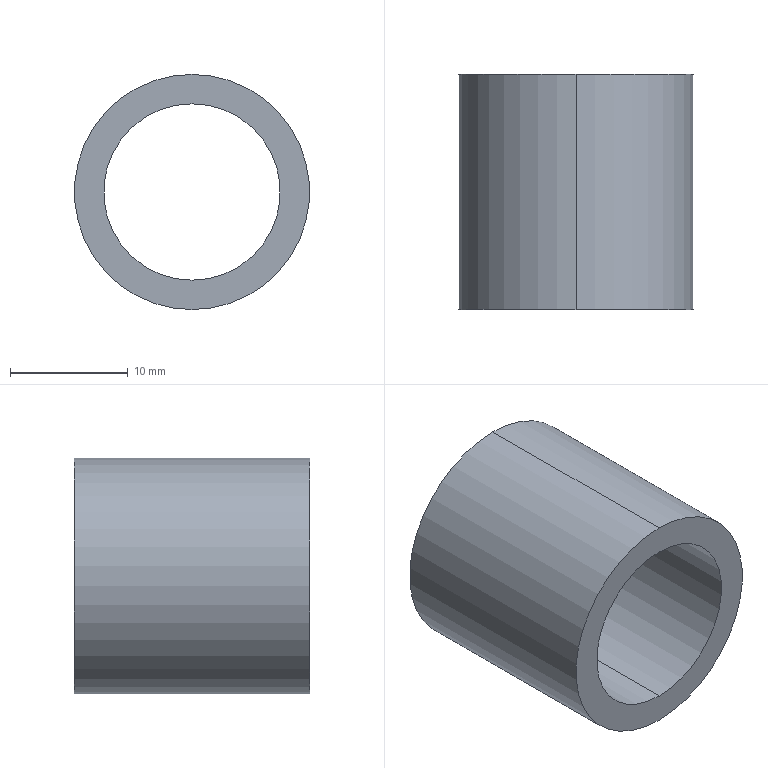Part | SolidWorks | features Extrusion 1 | 1 solid | 6 faces | box 20 x 20 x 20 mm | volume 2749 mm3 | cylinder 4 | plane 2 | commonest cylinder face diameters 15 x2 20 x2
STEP:
#1=CARTESIAN_POINT('',(0.,10.,-7.5));
#2=VERTEX_POINT('',#1);
#3=CARTESIAN_POINT('',(0.,10.,7.5));
#4=VERTEX_POINT('',#3);
#5=CARTESIAN_POINT('',(0.,10.,0.));
#6=DIRECTION('',(0.,1.,0.));
#7=DIRECTION('',(0.,0.,1.));
#8=AXIS2_PLACEMENT_3D('',#5,#6,#7);
#9=CIRCLE('',#8,7.5);
#10=EDGE_CURVE('',#2,#4,#9,.T.);
#11=ORIENTED_EDGE('',*,*,#10,.T.);
#12=CARTESIAN_POINT('',(0.,-10.,7.5));
#13=VERTEX_POINT('',#12);
#14=CARTESIAN_POINT('',(0.,10.,7.5));
#15=DIRECTION('',(0.,-1.,0.));
#16=VECTOR('',#15,1000.);
#17=LINE('',#14,#16);
#18=EDGE_CURVE('',#4,#13,#17,.T.);
#19=ORIENTED_EDGE('',*,*,#18,.T.);
#20=CARTESIAN_POINT('',(0.,-10.,-7.5));
#21=VERTEX_POINT('',#20);
#22=CARTESIAN_POINT('',(0.,-10.,0.));
#23=DIRECTION('',(0.,1.,0.));
#24=DIRECTION('',(0.,0.,1.));
#25=AXIS2_PLACEMENT_3D('',#22,#23,#24);
#26=CIRCLE('',#25,7.5);
#27=EDGE_CURVE('',#21,#13,#26,.T.);
#28=ORIENTED_EDGE('',*,*,#27,.F.);
#29=CARTESIAN_POINT('',(0.,10.,-7.5));
#30=DIRECTION('',(0.,-1.,0.));
#31=VECTOR('',#30,1000.);
#32=LINE('',#29,#31);
#33=EDGE_CURVE('',#2,#21,#32,.T.);
#34=ORIENTED_EDGE('',*,*,#33,.F.);
#35=EDGE_LOOP('',(#11,#19,#28,#34));
#36=FACE_OUTER_BOUND('',#35,.T.);
#37=CARTESIAN_POINT('',(0.,10.,0.));
#38=DIRECTION('',(0.,-1.,0.));
#39=DIRECTION('',(0.,0.,-1.));
#40=AXIS2_PLACEMENT_3D('',#37,#38,#39);
#41=CYLINDRICAL_SURFACE('',#40,7.5);
#42=ADVANCED_FACE('',(#36),#41,.F.);
#43=CARTESIAN_POINT('',(0.,10.,10.));
#44=VERTEX_POINT('',#43);
#45=CARTESIAN_POINT('',(0.,10.,-10.));
#46=VERTEX_POINT('',#45);
#47=CARTESIAN_POINT('',(0.,10.,0.));
#48=DIRECTION('',(0.,1.,0.));
#49=DIRECTION('',(0.,0.,1.));
#50=AXIS2_PLACEMENT_3D('',#47,#48,#49);
#51=CIRCLE('',#50,10.);
#52=EDGE_CURVE('',#44,#46,#51,.T.);
#53=ORIENTED_EDGE('',*,*,#52,.F.);
#54=CARTESIAN_POINT('',(0.,-10.,10.));
#55=VERTEX_POINT('',#54);
#56=CARTESIAN_POINT('',(0.,10.,10.));
#57=DIRECTION('',(0.,-1.,0.));
#58=VECTOR('',#57,1000.);
#59=LINE('',#56,#58);
#60=EDGE_CURVE('',#44,#55,#59,.T.);
#61=ORIENTED_EDGE('',*,*,#60,.T.);
#62=CARTESIAN_POINT('',(0.,-10.,-10.));
#63=VERTEX_POINT('',#62);
#64=CARTESIAN_POINT('',(0.,-10.,0.));
#65=DIRECTION('',(0.,1.,0.));
#66=DIRECTION('',(0.,0.,1.));
#67=AXIS2_PLACEMENT_3D('',#64,#65,#66);
#68=CIRCLE('',#67,10.);
#69=EDGE_CURVE('',#55,#63,#68,.T.);
#70=ORIENTED_EDGE('',*,*,#69,.T.);
#71=CARTESIAN_POINT('',(0.,10.,-10.));
#72=DIRECTION('',(0.,-1.,0.));
#73=VECTOR('',#72,1000.);
#74=LINE('',#71,#73);
#75=EDGE_CURVE('',#46,#63,#74,.T.);
#76=ORIENTED_EDGE('',*,*,#75,.F.);
#77=EDGE_LOOP('',(#53,#61,#70,#76));
#78=FACE_OUTER_BOUND('',#77,.T.);
#79=CARTESIAN_POINT('',(0.,10.,0.));
#80=DIRECTION('',(0.,-1.,0.));
#81=DIRECTION('',(0.,0.,-1.));
#82=AXIS2_PLACEMENT_3D('',#79,#80,#81);
#83=CYLINDRICAL_SURFACE('',#82,10.);
#84=ADVANCED_FACE('',(#78),#83,.T.);
#85=CARTESIAN_POINT('',(0.,10.,0.));
#86=DIRECTION('',(0.,1.,0.));
#87=DIRECTION('',(0.,0.,1.));
#88=AXIS2_PLACEMENT_3D('',#85,#86,#87);
#89=CIRCLE('',#88,10.);
#90=EDGE_CURVE('',#46,#44,#89,.T.);
#91=ORIENTED_EDGE('',*,*,#90,.T.);
#92=ORIENTED_EDGE('',*,*,#52,.T.);
#93=EDGE_LOOP('',(#91,#92));
#94=FACE_OUTER_BOUND('',#93,.T.);
#95=ORIENTED_EDGE('',*,*,#10,.F.);
#96=CARTESIAN_POINT('',(0.,10.,0.));
#97=DIRECTION('',(0.,1.,0.));
#98=DIRECTION('',(0.,0.,1.));
#99=AXIS2_PLACEMENT_3D('',#96,#97,#98);
#100=CIRCLE('',#99,7.5);
#101=EDGE_CURVE('',#4,#2,#100,.T.);
#102=ORIENTED_EDGE('',*,*,#101,.F.);
#103=EDGE_LOOP('',(#95,#102));
#104=FACE_BOUND('',#103,.T.);
#105=CARTESIAN_POINT('',(0.,10.,0.));
#106=DIRECTION('',(0.,1.,0.));
#107=DIRECTION('',(0.,0.,1.));
#108=AXIS2_PLACEMENT_3D('',#105,#106,#107);
#109=PLANE('',#108);
#110=ADVANCED_FACE('',(#94,#104),#109,.T.);
#111=CARTESIAN_POINT('',(0.,-10.,0.));
#112=DIRECTION('',(0.,1.,0.));
#113=DIRECTION('',(0.,0.,1.));
#114=AXIS2_PLACEMENT_3D('',#111,#112,#113);
#115=CIRCLE('',#114,10.);
#116=EDGE_CURVE('',#63,#55,#115,.T.);
#117=ORIENTED_EDGE('',*,*,#116,.F.);
#118=ORIENTED_EDGE('',*,*,#69,.F.);
#119=EDGE_LOOP('',(#117,#118));
#120=FACE_OUTER_BOUND('',#119,.T.);
#121=ORIENTED_EDGE('',*,*,#27,.T.);
#122=CARTESIAN_POINT('',(0.,-10.,0.));
#123=DIRECTION('',(0.,1.,0.));
#124=DIRECTION('',(0.,0.,1.));
#125=AXIS2_PLACEMENT_3D('',#122,#123,#124);
#126=CIRCLE('',#125,7.5);
#127=EDGE_CURVE('',#13,#21,#126,.T.);
#128=ORIENTED_EDGE('',*,*,#127,.T.);
#129=EDGE_LOOP('',(#121,#128));
#130=FACE_BOUND('',#129,.T.);
#131=CARTESIAN_POINT('',(0.,-10.,0.));
#132=DIRECTION('',(0.,1.,0.));
#133=DIRECTION('',(0.,0.,1.));
#134=AXIS2_PLACEMENT_3D('',#131,#132,#133);
#135=PLANE('',#134);
#136=ADVANCED_FACE('',(#120,#130),#135,.F.);
#137=ORIENTED_EDGE('',*,*,#60,.F.);
#138=ORIENTED_EDGE('',*,*,#90,.F.);
#139=ORIENTED_EDGE('',*,*,#75,.T.);
#140=ORIENTED_EDGE('',*,*,#116,.T.);
#141=EDGE_LOOP('',(#137,#138,#139,#140));
#142=FACE_OUTER_BOUND('',#141,.T.);
#143=CARTESIAN_POINT('',(0.,10.,0.));
#144=DIRECTION('',(0.,-1.,0.));
#145=DIRECTION('',(0.,0.,-1.));
#146=AXIS2_PLACEMENT_3D('',#143,#144,#145);
#147=CYLINDRICAL_SURFACE('',#146,10.);
#148=ADVANCED_FACE('',(#142),#147,.T.);
#149=ORIENTED_EDGE('',*,*,#18,.F.);
#150=ORIENTED_EDGE('',*,*,#101,.T.);
#151=ORIENTED_EDGE('',*,*,#33,.T.);
#152=ORIENTED_EDGE('',*,*,#127,.F.);
#153=EDGE_LOOP('',(#149,#150,#151,#152));
#154=FACE_OUTER_BOUND('',#153,.T.);
#155=CARTESIAN_POINT('',(0.,10.,0.));
#156=DIRECTION('',(0.,-1.,0.));
#157=DIRECTION('',(0.,0.,-1.));
#158=AXIS2_PLACEMENT_3D('',#155,#156,#157);
#159=CYLINDRICAL_SURFACE('',#158,7.5);
#160=ADVANCED_FACE('',(#154),#159,.F.);
#161=CLOSED_SHELL('',(#42,#84,#110,#136,#148,#160));
#162=MANIFOLD_SOLID_BREP('',#161);
#163=CARTESIAN_POINT('',(0.,0.,0.));
#164=DIRECTION('',(0.,0.,1.));
#165=DIRECTION('',(1.,0.,0.));
#166=AXIS2_PLACEMENT_3D('',#163,#164,#165);
#167=(LENGTH_UNIT()NAMED_UNIT(*)SI_UNIT(.MILLI.,.METRE.));
#168=UNCERTAINTY_MEASURE_WITH_UNIT(LENGTH_MEASURE(0.00001),#167,'','');
#169=(NAMED_UNIT(*)PLANE_ANGLE_UNIT()SI_UNIT($,.RADIAN.));
#170=(NAMED_UNIT(*)SI_UNIT($,.STERADIAN.)SOLID_ANGLE_UNIT());
#171=(GEOMETRIC_REPRESENTATION_CONTEXT(3)GLOBAL_UNCERTAINTY_ASSIGNED_CONTEXT((#168))GLOBAL_UNIT_ASSIGNED_CONTEXT((#167,#169,#170))REPRESENTATION_CONTEXT('',''));
#172=ADVANCED_BREP_SHAPE_REPRESENTATION('',(#162,#166),#171);